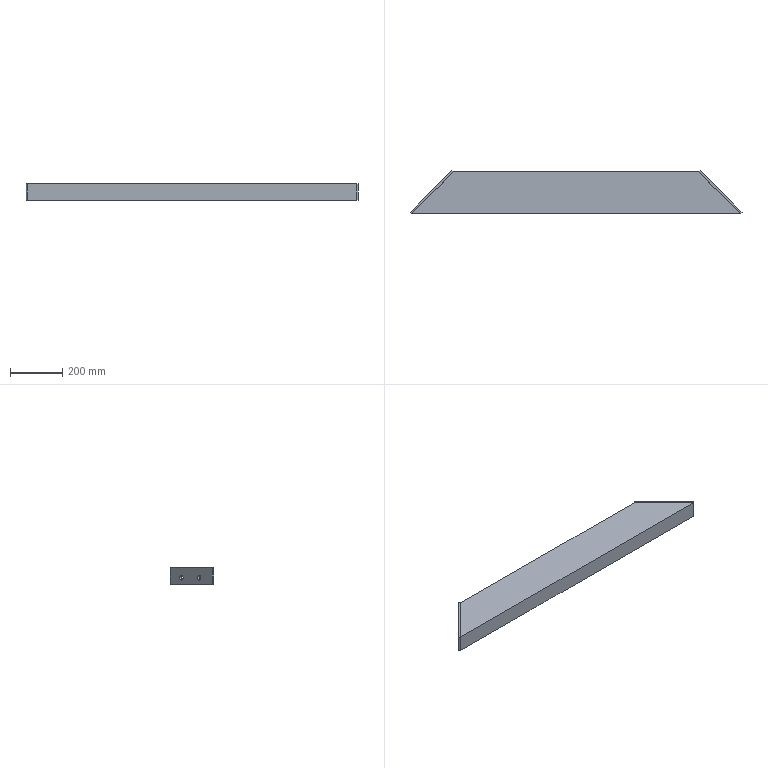Part | STEP file | PN_0010 stair platform brace 1257_Default<As Machined> | 3 solids | 30 faces | box 1268 x 165.463 x 63 mm | volume 2607828 mm3 | plane 22 | cylinder 8 | commonest cylinder face diameters 18 x4 10 x2 20 x2